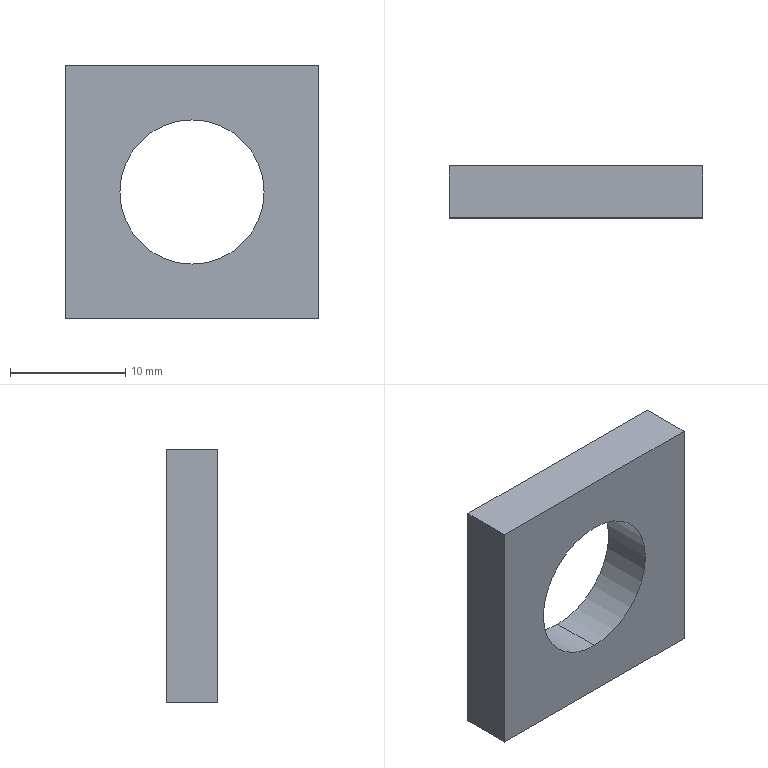Part | SolidWorks | features FlatPattern 1, SMBaseFlange 1, SheetMetal 1 | 1 solid | 8 faces | box 22 x 4.5 x 22 mm | volume 1626 mm3 | plane 6 | cylinder 2 | commonest cylinder face diameters 12.5 x2
STEP:
#1=CARTESIAN_POINT('',(0.,-4.5,-6.25));
#2=VERTEX_POINT('',#1);
#3=CARTESIAN_POINT('',(0.,-4.5,6.25));
#4=VERTEX_POINT('',#3);
#5=CARTESIAN_POINT('',(0.,-4.5,0.));
#6=DIRECTION('',(0.,1.,0.));
#7=DIRECTION('',(0.,0.,1.));
#8=AXIS2_PLACEMENT_3D('',#5,#6,#7);
#9=CIRCLE('',#8,6.25);
#10=EDGE_CURVE('',#2,#4,#9,.T.);
#11=ORIENTED_EDGE('',*,*,#10,.F.);
#12=CARTESIAN_POINT('',(0.,0.,-6.25));
#13=VERTEX_POINT('',#12);
#14=CARTESIAN_POINT('',(0.,-4.5,-6.25));
#15=DIRECTION('',(0.,1.,0.));
#16=VECTOR('',#15,1000.);
#17=LINE('',#14,#16);
#18=EDGE_CURVE('',#2,#13,#17,.T.);
#19=ORIENTED_EDGE('',*,*,#18,.T.);
#20=CARTESIAN_POINT('',(0.,0.,6.25));
#21=VERTEX_POINT('',#20);
#22=CARTESIAN_POINT('',(0.,0.,0.));
#23=DIRECTION('',(0.,1.,0.));
#24=DIRECTION('',(0.,0.,1.));
#25=AXIS2_PLACEMENT_3D('',#22,#23,#24);
#26=CIRCLE('',#25,6.25);
#27=EDGE_CURVE('',#13,#21,#26,.T.);
#28=ORIENTED_EDGE('',*,*,#27,.T.);
#29=CARTESIAN_POINT('',(0.,-4.5,6.25));
#30=DIRECTION('',(0.,1.,0.));
#31=VECTOR('',#30,1000.);
#32=LINE('',#29,#31);
#33=EDGE_CURVE('',#4,#21,#32,.T.);
#34=ORIENTED_EDGE('',*,*,#33,.F.);
#35=EDGE_LOOP('',(#11,#19,#28,#34));
#36=FACE_OUTER_BOUND('',#35,.T.);
#37=CARTESIAN_POINT('',(0.,-4.5,0.));
#38=DIRECTION('',(0.,1.,0.));
#39=DIRECTION('',(0.,0.,1.));
#40=AXIS2_PLACEMENT_3D('',#37,#38,#39);
#41=CYLINDRICAL_SURFACE('',#40,6.25);
#42=ADVANCED_FACE('',(#36),#41,.F.);
#43=CARTESIAN_POINT('',(11.,0.,11.));
#44=VERTEX_POINT('',#43);
#45=CARTESIAN_POINT('',(11.,0.,-11.));
#46=VERTEX_POINT('',#45);
#47=CARTESIAN_POINT('',(11.,0.,-11.));
#48=DIRECTION('',(0.,0.,-1.));
#49=VECTOR('',#48,1000.);
#50=LINE('',#47,#49);
#51=EDGE_CURVE('',#44,#46,#50,.T.);
#52=ORIENTED_EDGE('',*,*,#51,.F.);
#53=CARTESIAN_POINT('',(11.,-4.5,11.));
#54=VERTEX_POINT('',#53);
#55=CARTESIAN_POINT('',(11.,-4.5,11.));
#56=DIRECTION('',(0.,1.,0.));
#57=VECTOR('',#56,1000.);
#58=LINE('',#55,#57);
#59=EDGE_CURVE('',#54,#44,#58,.T.);
#60=ORIENTED_EDGE('',*,*,#59,.F.);
#61=CARTESIAN_POINT('',(11.,-4.5,-11.));
#62=VERTEX_POINT('',#61);
#63=CARTESIAN_POINT('',(11.,-4.5,-11.));
#64=DIRECTION('',(0.,0.,-1.));
#65=VECTOR('',#64,1000.);
#66=LINE('',#63,#65);
#67=EDGE_CURVE('',#54,#62,#66,.T.);
#68=ORIENTED_EDGE('',*,*,#67,.T.);
#69=CARTESIAN_POINT('',(11.,-4.5,-11.));
#70=DIRECTION('',(0.,1.,0.));
#71=VECTOR('',#70,1000.);
#72=LINE('',#69,#71);
#73=EDGE_CURVE('',#62,#46,#72,.T.);
#74=ORIENTED_EDGE('',*,*,#73,.T.);
#75=EDGE_LOOP('',(#52,#60,#68,#74));
#76=FACE_OUTER_BOUND('',#75,.T.);
#77=CARTESIAN_POINT('',(11.,-4.5,-11.));
#78=DIRECTION('',(1.,0.,0.));
#79=DIRECTION('',(0.,0.,-1.));
#80=AXIS2_PLACEMENT_3D('',#77,#78,#79);
#81=PLANE('',#80);
#82=ADVANCED_FACE('',(#76),#81,.T.);
#83=CARTESIAN_POINT('',(-11.,0.,11.));
#84=VERTEX_POINT('',#83);
#85=CARTESIAN_POINT('',(-11.,0.,11.));
#86=DIRECTION('',(1.,0.,0.));
#87=VECTOR('',#86,1000.);
#88=LINE('',#85,#87);
#89=EDGE_CURVE('',#84,#44,#88,.T.);
#90=ORIENTED_EDGE('',*,*,#89,.F.);
#91=CARTESIAN_POINT('',(-11.,-4.5,11.));
#92=VERTEX_POINT('',#91);
#93=CARTESIAN_POINT('',(-11.,-4.5,11.));
#94=DIRECTION('',(0.,1.,0.));
#95=VECTOR('',#94,1000.);
#96=LINE('',#93,#95);
#97=EDGE_CURVE('',#92,#84,#96,.T.);
#98=ORIENTED_EDGE('',*,*,#97,.F.);
#99=CARTESIAN_POINT('',(-11.,-4.5,11.));
#100=DIRECTION('',(1.,0.,0.));
#101=VECTOR('',#100,1000.);
#102=LINE('',#99,#101);
#103=EDGE_CURVE('',#92,#54,#102,.T.);
#104=ORIENTED_EDGE('',*,*,#103,.T.);
#105=ORIENTED_EDGE('',*,*,#59,.T.);
#106=EDGE_LOOP('',(#90,#98,#104,#105));
#107=FACE_OUTER_BOUND('',#106,.T.);
#108=CARTESIAN_POINT('',(-11.,-4.5,11.));
#109=DIRECTION('',(0.,0.,1.));
#110=DIRECTION('',(1.,0.,0.));
#111=AXIS2_PLACEMENT_3D('',#108,#109,#110);
#112=PLANE('',#111);
#113=ADVANCED_FACE('',(#107),#112,.T.);
#114=CARTESIAN_POINT('',(-11.,0.,-11.));
#115=VERTEX_POINT('',#114);
#116=CARTESIAN_POINT('',(-11.,0.,-11.));
#117=DIRECTION('',(0.,0.,1.));
#118=VECTOR('',#117,1000.);
#119=LINE('',#116,#118);
#120=EDGE_CURVE('',#115,#84,#119,.T.);
#121=ORIENTED_EDGE('',*,*,#120,.F.);
#122=CARTESIAN_POINT('',(-11.,-4.5,-11.));
#123=VERTEX_POINT('',#122);
#124=CARTESIAN_POINT('',(-11.,-4.5,-11.));
#125=DIRECTION('',(0.,1.,0.));
#126=VECTOR('',#125,1000.);
#127=LINE('',#124,#126);
#128=EDGE_CURVE('',#123,#115,#127,.T.);
#129=ORIENTED_EDGE('',*,*,#128,.F.);
#130=CARTESIAN_POINT('',(-11.,-4.5,-11.));
#131=DIRECTION('',(0.,0.,1.));
#132=VECTOR('',#131,1000.);
#133=LINE('',#130,#132);
#134=EDGE_CURVE('',#123,#92,#133,.T.);
#135=ORIENTED_EDGE('',*,*,#134,.T.);
#136=ORIENTED_EDGE('',*,*,#97,.T.);
#137=EDGE_LOOP('',(#121,#129,#135,#136));
#138=FACE_OUTER_BOUND('',#137,.T.);
#139=CARTESIAN_POINT('',(-11.,-4.5,-11.));
#140=DIRECTION('',(-1.,0.,0.));
#141=DIRECTION('',(0.,0.,1.));
#142=AXIS2_PLACEMENT_3D('',#139,#140,#141);
#143=PLANE('',#142);
#144=ADVANCED_FACE('',(#138),#143,.T.);
#145=CARTESIAN_POINT('',(-11.,0.,-11.));
#146=DIRECTION('',(-1.,0.,0.));
#147=VECTOR('',#146,1000.);
#148=LINE('',#145,#147);
#149=EDGE_CURVE('',#46,#115,#148,.T.);
#150=ORIENTED_EDGE('',*,*,#149,.F.);
#151=ORIENTED_EDGE('',*,*,#73,.F.);
#152=CARTESIAN_POINT('',(-11.,-4.5,-11.));
#153=DIRECTION('',(-1.,0.,0.));
#154=VECTOR('',#153,1000.);
#155=LINE('',#152,#154);
#156=EDGE_CURVE('',#62,#123,#155,.T.);
#157=ORIENTED_EDGE('',*,*,#156,.T.);
#158=ORIENTED_EDGE('',*,*,#128,.T.);
#159=EDGE_LOOP('',(#150,#151,#157,#158));
#160=FACE_OUTER_BOUND('',#159,.T.);
#161=CARTESIAN_POINT('',(-11.,-4.5,-11.));
#162=DIRECTION('',(0.,0.,-1.));
#163=DIRECTION('',(-1.,0.,0.));
#164=AXIS2_PLACEMENT_3D('',#161,#162,#163);
#165=PLANE('',#164);
#166=ADVANCED_FACE('',(#160),#165,.T.);
#167=CARTESIAN_POINT('',(0.,-4.5,0.));
#168=DIRECTION('',(0.,1.,0.));
#169=DIRECTION('',(0.,0.,1.));
#170=AXIS2_PLACEMENT_3D('',#167,#168,#169);
#171=CIRCLE('',#170,6.25);
#172=EDGE_CURVE('',#4,#2,#171,.T.);
#173=ORIENTED_EDGE('',*,*,#172,.T.);
#174=ORIENTED_EDGE('',*,*,#10,.T.);
#175=EDGE_LOOP('',(#173,#174));
#176=FACE_BOUND('',#175,.T.);
#177=ORIENTED_EDGE('',*,*,#67,.F.);
#178=ORIENTED_EDGE('',*,*,#103,.F.);
#179=ORIENTED_EDGE('',*,*,#134,.F.);
#180=ORIENTED_EDGE('',*,*,#156,.F.);
#181=EDGE_LOOP('',(#177,#178,#179,#180));
#182=FACE_OUTER_BOUND('',#181,.T.);
#183=CARTESIAN_POINT('',(0.,-4.5,0.));
#184=DIRECTION('',(0.,1.,0.));
#185=DIRECTION('',(0.,0.,1.));
#186=AXIS2_PLACEMENT_3D('',#183,#184,#185);
#187=PLANE('',#186);
#188=ADVANCED_FACE('',(#176,#182),#187,.F.);
#189=CARTESIAN_POINT('',(0.,0.,0.));
#190=DIRECTION('',(0.,1.,0.));
#191=DIRECTION('',(0.,0.,1.));
#192=AXIS2_PLACEMENT_3D('',#189,#190,#191);
#193=CIRCLE('',#192,6.25);
#194=EDGE_CURVE('',#21,#13,#193,.T.);
#195=ORIENTED_EDGE('',*,*,#194,.F.);
#196=ORIENTED_EDGE('',*,*,#27,.F.);
#197=EDGE_LOOP('',(#195,#196));
#198=FACE_BOUND('',#197,.T.);
#199=ORIENTED_EDGE('',*,*,#51,.T.);
#200=ORIENTED_EDGE('',*,*,#149,.T.);
#201=ORIENTED_EDGE('',*,*,#120,.T.);
#202=ORIENTED_EDGE('',*,*,#89,.T.);
#203=EDGE_LOOP('',(#199,#200,#201,#202));
#204=FACE_OUTER_BOUND('',#203,.T.);
#205=CARTESIAN_POINT('',(0.,0.,0.));
#206=DIRECTION('',(0.,1.,0.));
#207=DIRECTION('',(0.,0.,1.));
#208=AXIS2_PLACEMENT_3D('',#205,#206,#207);
#209=PLANE('',#208);
#210=ADVANCED_FACE('',(#198,#204),#209,.T.);
#211=ORIENTED_EDGE('',*,*,#18,.F.);
#212=ORIENTED_EDGE('',*,*,#172,.F.);
#213=ORIENTED_EDGE('',*,*,#33,.T.);
#214=ORIENTED_EDGE('',*,*,#194,.T.);
#215=EDGE_LOOP('',(#211,#212,#213,#214));
#216=FACE_OUTER_BOUND('',#215,.T.);
#217=CARTESIAN_POINT('',(0.,-4.5,0.));
#218=DIRECTION('',(0.,1.,0.));
#219=DIRECTION('',(0.,0.,1.));
#220=AXIS2_PLACEMENT_3D('',#217,#218,#219);
#221=CYLINDRICAL_SURFACE('',#220,6.25);
#222=ADVANCED_FACE('',(#216),#221,.F.);
#223=CLOSED_SHELL('',(#42,#82,#113,#144,#166,#188,#210,#222));
#224=MANIFOLD_SOLID_BREP('',#223);
#225=CARTESIAN_POINT('',(0.,0.,0.));
#226=DIRECTION('',(0.,0.,1.));
#227=DIRECTION('',(1.,0.,0.));
#228=AXIS2_PLACEMENT_3D('',#225,#226,#227);
#229=(LENGTH_UNIT()NAMED_UNIT(*)SI_UNIT(.MILLI.,.METRE.));
#230=UNCERTAINTY_MEASURE_WITH_UNIT(LENGTH_MEASURE(0.00001),#229,'','');
#231=(NAMED_UNIT(*)PLANE_ANGLE_UNIT()SI_UNIT($,.RADIAN.));
#232=(NAMED_UNIT(*)SI_UNIT($,.STERADIAN.)SOLID_ANGLE_UNIT());
#233=(GEOMETRIC_REPRESENTATION_CONTEXT(3)GLOBAL_UNCERTAINTY_ASSIGNED_CONTEXT((#230))GLOBAL_UNIT_ASSIGNED_CONTEXT((#229,#231,#232))REPRESENTATION_CONTEXT('',''));
#234=ADVANCED_BREP_SHAPE_REPRESENTATION('',(#224,#228),#233);